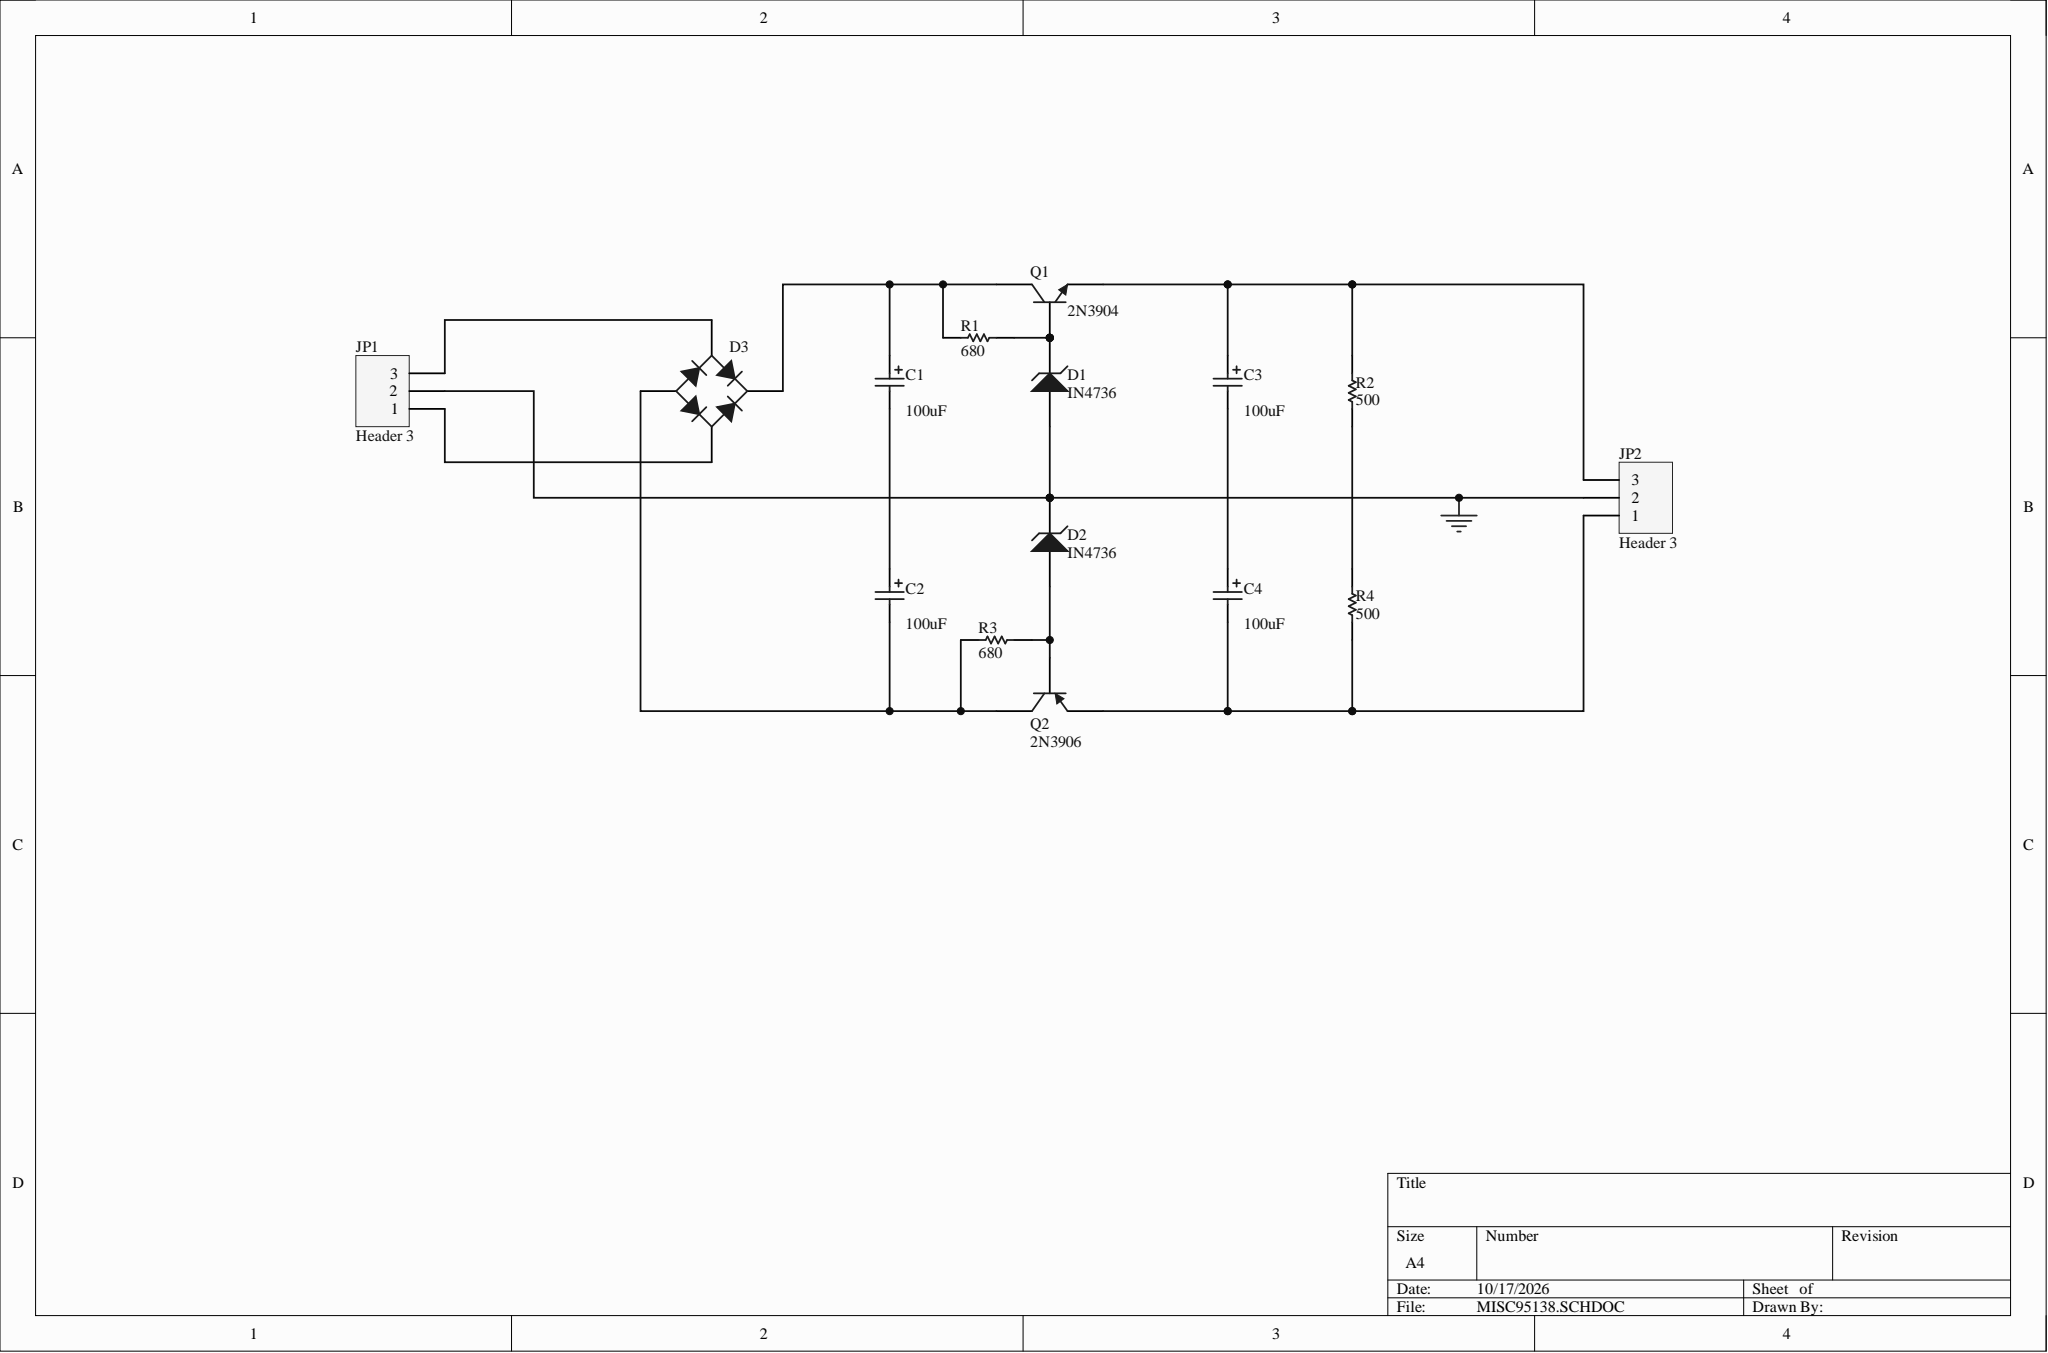Circuit board | Altium Designer | 15 parts | 12 nets
Bill of materials:
Comment,Description,Designator,Footprint,LibRef,Quantity
"Cap Pol1","Polarized Capacitor (Radial)","C1, C2, C3, C4","RB7.6-15","Cap Pol1","4"
"IN4736","Zener Diode","D1, D2","DIODE-0.7","D Zener","2"
"Bridge1","Full Wave Diode Bridge","D3","E-BIP-P4/D10","Bridge1","1"
"Header 3","Header, 3-Pin","JP1, JP2","HDR1X3","Header 3","2"
"2N3904","NPN General Purpose Amplifier","Q1","BCY-W3/E4","2N3904","1"
"2N3906","PNP General Purpose Amplifier","Q2","BCY-W3/E4","2N3906","1"
"Res1","Resistor","R1, R2, R3, R4","AXIAL-0.3","Res1","4"
Netlist (Protel format):
[
C1
RB7.6-15
Cap Pol1



]
[
C2
RB7.6-15
Cap Pol1



]
[
C3
RB7.6-15
Cap Pol1



]
[
C4
RB7.6-15
Cap Pol1



]
[
D1
DIODE-0.7
IN4736



]
[
D2
DIODE-0.7
IN4736



]
[
D3
E-BIP-P4/D10
Bridge1



]
[
JP1
HDR1X3
Header 3



]
[
JP2
HDR1X3
Header 3



]
[
Q1
BCY-W3/E4
2N3904



]
[
Q2
BCY-W3/E4
2N3906



]
[
R1
AXIAL-0.3
Res1



]
[
R2
AXIAL-0.3
Res1



]
[
R3
AXIAL-0.3
Res1



]
[
R4
AXIAL-0.3
Res1



]
(
NetR2_1
R2-1
R4-2
)
(
NetD3_4
D3-4
JP1-1
)
(
NetD3_2
D3-2
JP1-3
)
(
NetD2_1
D2-1
Q2-2
R3-2
)
(
NetD1_2
D1-2
Q1-2
R1-2
)
(
NetC4_2
C4-2
JP2-1
Q2-1
R4-1
)
(
NetC3_2
C3-2
C4-1
)
(
NetC3_1
C3-1
JP2-3
Q1-1
R2-2
)
(
NetC2_2
C2-2
D3-1
Q2-3
R3-1
)
(
NetC1_2
C1-2
C2-1
)
(
NetC1_1
C1-1
D3-3
Q1-3
R1-1
)
(
GND
D1-1
D2-2
JP1-2
JP2-2
)